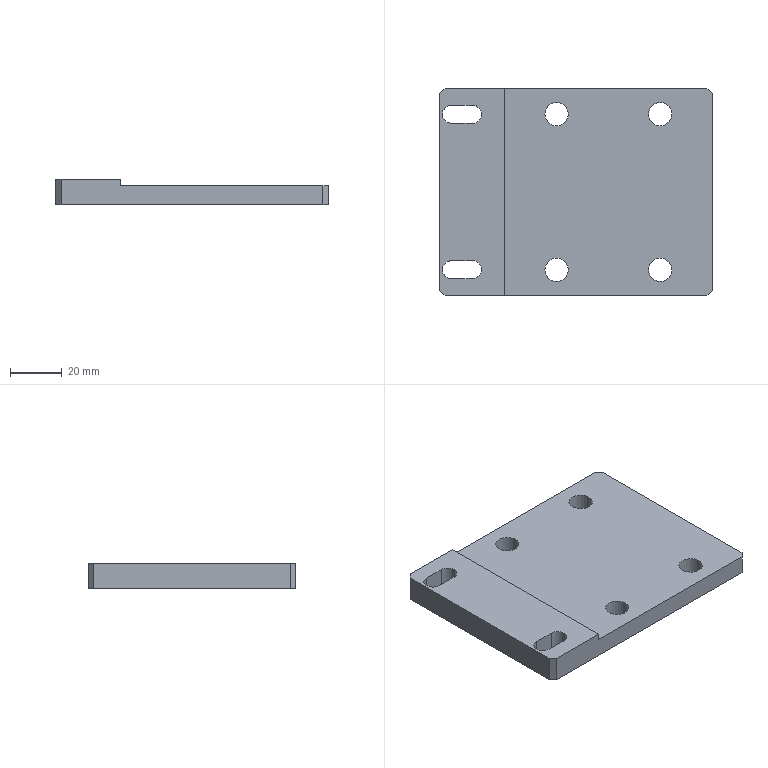Part | SolidWorks | features HoleWzd 2, ICE 2, Chamfer 1, Extrusion 1, LPattern 1 | 1 solid | 30 faces | box 105 x 80 x 10 mm | volume 64132 mm3 | plane 16 | cylinder 14 | commonest cylinder face diameters 9 x8 7 x6
STEP:
#1=CARTESIAN_POINT('',(-36.5,-30.,-5.));
#2=VERTEX_POINT('',#1);
#3=CARTESIAN_POINT('',(-40.,-26.5,-5.));
#4=VERTEX_POINT('',#3);
#5=CARTESIAN_POINT('',(-40.,-30.,-5.));
#6=DIRECTION('',(0.,0.,1.));
#7=DIRECTION('',(1.,0.,0.));
#8=AXIS2_PLACEMENT_3D('',#5,#6,#7);
#9=CIRCLE('',#8,3.5);
#10=EDGE_CURVE('',#2,#4,#9,.T.);
#11=ORIENTED_EDGE('',*,*,#10,.F.);
#12=CARTESIAN_POINT('',(-36.5,-30.,5.));
#13=VERTEX_POINT('',#12);
#14=CARTESIAN_POINT('',(-36.5,-30.,-5.));
#15=DIRECTION('',(0.,0.,1.));
#16=VECTOR('',#15,1000.);
#17=LINE('',#14,#16);
#18=EDGE_CURVE('',#2,#13,#17,.T.);
#19=ORIENTED_EDGE('',*,*,#18,.T.);
#20=CARTESIAN_POINT('',(-40.,-26.5,5.));
#21=VERTEX_POINT('',#20);
#22=CARTESIAN_POINT('',(-40.,-30.,5.));
#23=DIRECTION('',(0.,0.,1.));
#24=DIRECTION('',(1.,0.,0.));
#25=AXIS2_PLACEMENT_3D('',#22,#23,#24);
#26=CIRCLE('',#25,3.5);
#27=EDGE_CURVE('',#13,#21,#26,.T.);
#28=ORIENTED_EDGE('',*,*,#27,.T.);
#29=CARTESIAN_POINT('',(-40.,-26.5,-5.));
#30=DIRECTION('',(0.,0.,1.));
#31=VECTOR('',#30,1000.);
#32=LINE('',#29,#31);
#33=EDGE_CURVE('',#4,#21,#32,.T.);
#34=ORIENTED_EDGE('',*,*,#33,.F.);
#35=EDGE_LOOP('',(#11,#19,#28,#34));
#36=FACE_OUTER_BOUND('',#35,.T.);
#37=CARTESIAN_POINT('',(-40.,-30.,-5.));
#38=DIRECTION('',(0.,0.,1.));
#39=DIRECTION('',(1.,0.,0.));
#40=AXIS2_PLACEMENT_3D('',#37,#38,#39);
#41=CYLINDRICAL_SURFACE('',#40,3.5);
#42=ADVANCED_FACE('',(#36),#41,.F.);
#43=CARTESIAN_POINT('',(-36.5,30.,-5.));
#44=VERTEX_POINT('',#43);
#45=CARTESIAN_POINT('',(-40.,33.5,-5.));
#46=VERTEX_POINT('',#45);
#47=CARTESIAN_POINT('',(-40.,30.,-5.));
#48=DIRECTION('',(0.,0.,1.));
#49=DIRECTION('',(1.,0.,0.));
#50=AXIS2_PLACEMENT_3D('',#47,#48,#49);
#51=CIRCLE('',#50,3.5);
#52=EDGE_CURVE('',#44,#46,#51,.T.);
#53=ORIENTED_EDGE('',*,*,#52,.F.);
#54=CARTESIAN_POINT('',(-36.5,30.,5.));
#55=VERTEX_POINT('',#54);
#56=CARTESIAN_POINT('',(-36.5,30.,-5.));
#57=DIRECTION('',(0.,0.,1.));
#58=VECTOR('',#57,1000.);
#59=LINE('',#56,#58);
#60=EDGE_CURVE('',#44,#55,#59,.T.);
#61=ORIENTED_EDGE('',*,*,#60,.T.);
#62=CARTESIAN_POINT('',(-40.,33.5,5.));
#63=VERTEX_POINT('',#62);
#64=CARTESIAN_POINT('',(-40.,30.,5.));
#65=DIRECTION('',(0.,0.,1.));
#66=DIRECTION('',(1.,0.,0.));
#67=AXIS2_PLACEMENT_3D('',#64,#65,#66);
#68=CIRCLE('',#67,3.5);
#69=EDGE_CURVE('',#55,#63,#68,.T.);
#70=ORIENTED_EDGE('',*,*,#69,.T.);
#71=CARTESIAN_POINT('',(-40.,33.5,-5.));
#72=DIRECTION('',(0.,0.,1.));
#73=VECTOR('',#72,1000.);
#74=LINE('',#71,#73);
#75=EDGE_CURVE('',#46,#63,#74,.T.);
#76=ORIENTED_EDGE('',*,*,#75,.F.);
#77=EDGE_LOOP('',(#53,#61,#70,#76));
#78=FACE_OUTER_BOUND('',#77,.T.);
#79=CARTESIAN_POINT('',(-40.,30.,-5.));
#80=DIRECTION('',(0.,0.,1.));
#81=DIRECTION('',(1.,0.,0.));
#82=AXIS2_PLACEMENT_3D('',#79,#80,#81);
#83=CYLINDRICAL_SURFACE('',#82,3.5);
#84=ADVANCED_FACE('',(#78),#83,.F.);
#85=CARTESIAN_POINT('',(-12.,30.,-5.));
#86=VERTEX_POINT('',#85);
#87=CARTESIAN_POINT('',(-3.,30.,-5.));
#88=VERTEX_POINT('',#87);
#89=CARTESIAN_POINT('',(-7.5,30.,-5.));
#90=DIRECTION('',(0.,0.,1.));
#91=DIRECTION('',(1.,0.,0.));
#92=AXIS2_PLACEMENT_3D('',#89,#90,#91);
#93=CIRCLE('',#92,4.5);
#94=EDGE_CURVE('',#86,#88,#93,.T.);
#95=ORIENTED_EDGE('',*,*,#94,.F.);
#96=CARTESIAN_POINT('',(-12.,30.,2.5));
#97=VERTEX_POINT('',#96);
#98=CARTESIAN_POINT('',(-12.,30.,5.));
#99=DIRECTION('',(0.,0.,1.));
#100=VECTOR('',#99,1000.);
#101=LINE('',#98,#100);
#102=EDGE_CURVE('',#86,#97,#101,.T.);
#103=ORIENTED_EDGE('',*,*,#102,.T.);
#104=CARTESIAN_POINT('',(-3.,30.,2.5));
#105=VERTEX_POINT('',#104);
#106=CARTESIAN_POINT('',(-7.5,30.,2.5));
#107=DIRECTION('',(0.,0.,-1.));
#108=DIRECTION('',(-1.,0.,0.));
#109=AXIS2_PLACEMENT_3D('',#106,#107,#108);
#110=CIRCLE('',#109,4.5);
#111=EDGE_CURVE('',#105,#97,#110,.T.);
#112=ORIENTED_EDGE('',*,*,#111,.F.);
#113=CARTESIAN_POINT('',(-3.,30.,5.));
#114=DIRECTION('',(0.,0.,1.));
#115=VECTOR('',#114,1000.);
#116=LINE('',#113,#115);
#117=EDGE_CURVE('',#88,#105,#116,.T.);
#118=ORIENTED_EDGE('',*,*,#117,.F.);
#119=EDGE_LOOP('',(#95,#103,#112,#118));
#120=FACE_OUTER_BOUND('',#119,.T.);
#121=CARTESIAN_POINT('',(-7.5,30.,5.));
#122=DIRECTION('',(0.,0.,1.));
#123=DIRECTION('',(1.,0.,0.));
#124=AXIS2_PLACEMENT_3D('',#121,#122,#123);
#125=CYLINDRICAL_SURFACE('',#124,4.5);
#126=ADVANCED_FACE('',(#120),#125,.F.);
#127=CARTESIAN_POINT('',(28.,30.,-5.));
#128=VERTEX_POINT('',#127);
#129=CARTESIAN_POINT('',(37.,30.,-5.));
#130=VERTEX_POINT('',#129);
#131=CARTESIAN_POINT('',(32.5,30.,-5.));
#132=DIRECTION('',(0.,0.,1.));
#133=DIRECTION('',(1.,0.,0.));
#134=AXIS2_PLACEMENT_3D('',#131,#132,#133);
#135=CIRCLE('',#134,4.5);
#136=EDGE_CURVE('',#128,#130,#135,.T.);
#137=ORIENTED_EDGE('',*,*,#136,.F.);
#138=CARTESIAN_POINT('',(28.,30.,2.5));
#139=VERTEX_POINT('',#138);
#140=CARTESIAN_POINT('',(28.,30.,5.));
#141=DIRECTION('',(0.,0.,1.));
#142=VECTOR('',#141,1000.);
#143=LINE('',#140,#142);
#144=EDGE_CURVE('',#128,#139,#143,.T.);
#145=ORIENTED_EDGE('',*,*,#144,.T.);
#146=CARTESIAN_POINT('',(37.,30.,2.5));
#147=VERTEX_POINT('',#146);
#148=CARTESIAN_POINT('',(32.5,30.,2.5));
#149=DIRECTION('',(0.,0.,-1.));
#150=DIRECTION('',(-1.,0.,0.));
#151=AXIS2_PLACEMENT_3D('',#148,#149,#150);
#152=CIRCLE('',#151,4.5);
#153=EDGE_CURVE('',#147,#139,#152,.T.);
#154=ORIENTED_EDGE('',*,*,#153,.F.);
#155=CARTESIAN_POINT('',(37.,30.,5.));
#156=DIRECTION('',(0.,0.,1.));
#157=VECTOR('',#156,1000.);
#158=LINE('',#155,#157);
#159=EDGE_CURVE('',#130,#147,#158,.T.);
#160=ORIENTED_EDGE('',*,*,#159,.F.);
#161=EDGE_LOOP('',(#137,#145,#154,#160));
#162=FACE_OUTER_BOUND('',#161,.T.);
#163=CARTESIAN_POINT('',(32.5,30.,5.));
#164=DIRECTION('',(0.,0.,1.));
#165=DIRECTION('',(1.,0.,0.));
#166=AXIS2_PLACEMENT_3D('',#163,#164,#165);
#167=CYLINDRICAL_SURFACE('',#166,4.5);
#168=ADVANCED_FACE('',(#162),#167,.F.);
#169=CARTESIAN_POINT('',(28.,-30.,-5.));
#170=VERTEX_POINT('',#169);
#171=CARTESIAN_POINT('',(37.,-30.,-5.));
#172=VERTEX_POINT('',#171);
#173=CARTESIAN_POINT('',(32.5,-30.,-5.));
#174=DIRECTION('',(0.,0.,1.));
#175=DIRECTION('',(1.,0.,0.));
#176=AXIS2_PLACEMENT_3D('',#173,#174,#175);
#177=CIRCLE('',#176,4.5);
#178=EDGE_CURVE('',#170,#172,#177,.T.);
#179=ORIENTED_EDGE('',*,*,#178,.F.);
#180=CARTESIAN_POINT('',(28.,-30.,2.5));
#181=VERTEX_POINT('',#180);
#182=CARTESIAN_POINT('',(28.,-30.,5.));
#183=DIRECTION('',(0.,0.,1.));
#184=VECTOR('',#183,1000.);
#185=LINE('',#182,#184);
#186=EDGE_CURVE('',#170,#181,#185,.T.);
#187=ORIENTED_EDGE('',*,*,#186,.T.);
#188=CARTESIAN_POINT('',(37.,-30.,2.5));
#189=VERTEX_POINT('',#188);
#190=CARTESIAN_POINT('',(32.5,-30.,2.5));
#191=DIRECTION('',(0.,0.,-1.));
#192=DIRECTION('',(-1.,0.,0.));
#193=AXIS2_PLACEMENT_3D('',#190,#191,#192);
#194=CIRCLE('',#193,4.5);
#195=EDGE_CURVE('',#189,#181,#194,.T.);
#196=ORIENTED_EDGE('',*,*,#195,.F.);
#197=CARTESIAN_POINT('',(37.,-30.,5.));
#198=DIRECTION('',(0.,0.,1.));
#199=VECTOR('',#198,1000.);
#200=LINE('',#197,#199);
#201=EDGE_CURVE('',#172,#189,#200,.T.);
#202=ORIENTED_EDGE('',*,*,#201,.F.);
#203=EDGE_LOOP('',(#179,#187,#196,#202));
#204=FACE_OUTER_BOUND('',#203,.T.);
#205=CARTESIAN_POINT('',(32.5,-30.,5.));
#206=DIRECTION('',(0.,0.,1.));
#207=DIRECTION('',(1.,0.,0.));
#208=AXIS2_PLACEMENT_3D('',#205,#206,#207);
#209=CYLINDRICAL_SURFACE('',#208,4.5);
#210=ADVANCED_FACE('',(#204),#209,.F.);
#211=CARTESIAN_POINT('',(-12.,-30.,-5.));
#212=VERTEX_POINT('',#211);
#213=CARTESIAN_POINT('',(-3.,-30.,-5.));
#214=VERTEX_POINT('',#213);
#215=CARTESIAN_POINT('',(-7.5,-30.,-5.));
#216=DIRECTION('',(0.,0.,1.));
#217=DIRECTION('',(1.,0.,0.));
#218=AXIS2_PLACEMENT_3D('',#215,#216,#217);
#219=CIRCLE('',#218,4.5);
#220=EDGE_CURVE('',#212,#214,#219,.T.);
#221=ORIENTED_EDGE('',*,*,#220,.F.);
#222=CARTESIAN_POINT('',(-12.,-30.,2.5));
#223=VERTEX_POINT('',#222);
#224=CARTESIAN_POINT('',(-12.,-30.,5.));
#225=DIRECTION('',(0.,0.,1.));
#226=VECTOR('',#225,1000.);
#227=LINE('',#224,#226);
#228=EDGE_CURVE('',#212,#223,#227,.T.);
#229=ORIENTED_EDGE('',*,*,#228,.T.);
#230=CARTESIAN_POINT('',(-3.,-30.,2.5));
#231=VERTEX_POINT('',#230);
#232=CARTESIAN_POINT('',(-7.5,-30.,2.5));
#233=DIRECTION('',(0.,0.,-1.));
#234=DIRECTION('',(-1.,0.,0.));
#235=AXIS2_PLACEMENT_3D('',#232,#233,#234);
#236=CIRCLE('',#235,4.5);
#237=EDGE_CURVE('',#231,#223,#236,.T.);
#238=ORIENTED_EDGE('',*,*,#237,.F.);
#239=CARTESIAN_POINT('',(-3.,-30.,5.));
#240=DIRECTION('',(0.,0.,1.));
#241=VECTOR('',#240,1000.);
#242=LINE('',#239,#241);
#243=EDGE_CURVE('',#214,#231,#242,.T.);
#244=ORIENTED_EDGE('',*,*,#243,.F.);
#245=EDGE_LOOP('',(#221,#229,#238,#244));
#246=FACE_OUTER_BOUND('',#245,.T.);
#247=CARTESIAN_POINT('',(-7.5,-30.,5.));
#248=DIRECTION('',(0.,0.,1.));
#249=DIRECTION('',(1.,0.,0.));
#250=AXIS2_PLACEMENT_3D('',#247,#248,#249);
#251=CYLINDRICAL_SURFACE('',#250,4.5);
#252=ADVANCED_FACE('',(#246),#251,.F.);
#253=CARTESIAN_POINT('',(52.5,-38.,-5.));
#254=VERTEX_POINT('',#253);
#255=CARTESIAN_POINT('',(52.5,38.,-5.));
#256=VERTEX_POINT('',#255);
#257=CARTESIAN_POINT('',(52.5,40.,-5.));
#258=DIRECTION('',(0.,1.,0.));
#259=VECTOR('',#258,1000.);
#260=LINE('',#257,#259);
#261=EDGE_CURVE('',#254,#256,#260,.T.);
#262=ORIENTED_EDGE('',*,*,#261,.T.);
#263=CARTESIAN_POINT('',(52.5,38.,2.5));
#264=VERTEX_POINT('',#263);
#265=CARTESIAN_POINT('',(52.5,38.,5.));
#266=DIRECTION('',(0.,0.,1.));
#267=VECTOR('',#266,1000.);
#268=LINE('',#265,#267);
#269=EDGE_CURVE('',#256,#264,#268,.T.);
#270=ORIENTED_EDGE('',*,*,#269,.T.);
#271=CARTESIAN_POINT('',(52.5,-38.,2.5));
#272=VERTEX_POINT('',#271);
#273=CARTESIAN_POINT('',(52.5,40.,2.5));
#274=DIRECTION('',(0.,1.,0.));
#275=VECTOR('',#274,1000.);
#276=LINE('',#273,#275);
#277=EDGE_CURVE('',#272,#264,#276,.T.);
#278=ORIENTED_EDGE('',*,*,#277,.F.);
#279=CARTESIAN_POINT('',(52.5,-38.,5.));
#280=DIRECTION('',(0.,0.,-1.));
#281=VECTOR('',#280,1000.);
#282=LINE('',#279,#281);
#283=EDGE_CURVE('',#272,#254,#282,.T.);
#284=ORIENTED_EDGE('',*,*,#283,.T.);
#285=EDGE_LOOP('',(#262,#270,#278,#284));
#286=FACE_OUTER_BOUND('',#285,.T.);
#287=CARTESIAN_POINT('',(52.5,40.,5.));
#288=DIRECTION('',(-1.,0.,0.));
#289=DIRECTION('',(0.,-1.,0.));
#290=AXIS2_PLACEMENT_3D('',#287,#288,#289);
#291=PLANE('',#290);
#292=ADVANCED_FACE('',(#286),#291,.F.);
#293=CARTESIAN_POINT('',(50.5,40.,-5.));
#294=VERTEX_POINT('',#293);
#295=CARTESIAN_POINT('',(-50.5,40.,-5.));
#296=VERTEX_POINT('',#295);
#297=CARTESIAN_POINT('',(-52.5,40.,-5.));
#298=DIRECTION('',(-1.,0.,0.));
#299=VECTOR('',#298,1000.);
#300=LINE('',#297,#299);
#301=EDGE_CURVE('',#294,#296,#300,.T.);
#302=ORIENTED_EDGE('',*,*,#301,.T.);
#303=CARTESIAN_POINT('',(-50.5,40.,5.));
#304=VERTEX_POINT('',#303);
#305=CARTESIAN_POINT('',(-50.5,40.,5.));
#306=DIRECTION('',(0.,0.,1.));
#307=VECTOR('',#306,1000.);
#308=LINE('',#305,#307);
#309=EDGE_CURVE('',#296,#304,#308,.T.);
#310=ORIENTED_EDGE('',*,*,#309,.T.);
#311=CARTESIAN_POINT('',(-27.5,40.,5.));
#312=VERTEX_POINT('',#311);
#313=CARTESIAN_POINT('',(-52.5,40.,5.));
#314=DIRECTION('',(-1.,0.,0.));
#315=VECTOR('',#314,1000.);
#316=LINE('',#313,#315);
#317=EDGE_CURVE('',#312,#304,#316,.T.);
#318=ORIENTED_EDGE('',*,*,#317,.F.);
#319=CARTESIAN_POINT('',(-27.5,40.,2.5));
#320=VERTEX_POINT('',#319);
#321=CARTESIAN_POINT('',(-27.5,40.,2.5));
#322=DIRECTION('',(0.,0.,1.));
#323=VECTOR('',#322,1000.);
#324=LINE('',#321,#323);
#325=EDGE_CURVE('',#320,#312,#324,.T.);
#326=ORIENTED_EDGE('',*,*,#325,.F.);
#327=CARTESIAN_POINT('',(50.5,40.,2.5));
#328=VERTEX_POINT('',#327);
#329=CARTESIAN_POINT('',(52.5,40.,2.5));
#330=DIRECTION('',(-1.,0.,0.));
#331=VECTOR('',#330,1000.);
#332=LINE('',#329,#331);
#333=EDGE_CURVE('',#328,#320,#332,.T.);
#334=ORIENTED_EDGE('',*,*,#333,.F.);
#335=CARTESIAN_POINT('',(50.5,40.,5.));
#336=DIRECTION('',(0.,0.,-1.));
#337=VECTOR('',#336,1000.);
#338=LINE('',#335,#337);
#339=EDGE_CURVE('',#328,#294,#338,.T.);
#340=ORIENTED_EDGE('',*,*,#339,.T.);
#341=EDGE_LOOP('',(#302,#310,#318,#326,#334,#340));
#342=FACE_OUTER_BOUND('',#341,.T.);
#343=CARTESIAN_POINT('',(-52.5,40.,5.));
#344=DIRECTION('',(0.,-1.,0.));
#345=DIRECTION('',(0.,0.,-1.));
#346=AXIS2_PLACEMENT_3D('',#343,#344,#345);
#347=PLANE('',#346);
#348=ADVANCED_FACE('',(#342),#347,.F.);
#349=CARTESIAN_POINT('',(-52.5,38.,-5.));
#350=VERTEX_POINT('',#349);
#351=CARTESIAN_POINT('',(-52.5,-38.,-5.));
#352=VERTEX_POINT('',#351);
#353=CARTESIAN_POINT('',(-52.5,40.,-5.));
#354=DIRECTION('',(0.,-1.,0.));
#355=VECTOR('',#354,1000.);
#356=LINE('',#353,#355);
#357=EDGE_CURVE('',#350,#352,#356,.T.);
#358=ORIENTED_EDGE('',*,*,#357,.T.);
#359=CARTESIAN_POINT('',(-52.5,-38.,5.));
#360=VERTEX_POINT('',#359);
#361=CARTESIAN_POINT('',(-52.5,-38.,5.));
#362=DIRECTION('',(0.,0.,1.));
#363=VECTOR('',#362,1000.);
#364=LINE('',#361,#363);
#365=EDGE_CURVE('',#352,#360,#364,.T.);
#366=ORIENTED_EDGE('',*,*,#365,.T.);
#367=CARTESIAN_POINT('',(-52.5,38.,5.));
#368=VERTEX_POINT('',#367);
#369=CARTESIAN_POINT('',(-52.5,40.,5.));
#370=DIRECTION('',(0.,-1.,0.));
#371=VECTOR('',#370,1000.);
#372=LINE('',#369,#371);
#373=EDGE_CURVE('',#368,#360,#372,.T.);
#374=ORIENTED_EDGE('',*,*,#373,.F.);
#375=CARTESIAN_POINT('',(-52.5,38.,5.));
#376=DIRECTION('',(0.,0.,-1.));
#377=VECTOR('',#376,1000.);
#378=LINE('',#375,#377);
#379=EDGE_CURVE('',#368,#350,#378,.T.);
#380=ORIENTED_EDGE('',*,*,#379,.T.);
#381=EDGE_LOOP('',(#358,#366,#374,#380));
#382=FACE_OUTER_BOUND('',#381,.T.);
#383=CARTESIAN_POINT('',(-52.5,40.,5.));
#384=DIRECTION('',(1.,0.,0.));
#385=DIRECTION('',(0.,1.,0.));
#386=AXIS2_PLACEMENT_3D('',#383,#384,#385);
#387=PLANE('',#386);
#388=ADVANCED_FACE('',(#382),#387,.F.);
#389=CARTESIAN_POINT('',(-50.5,-40.,5.));
#390=VERTEX_POINT('',#389);
#391=CARTESIAN_POINT('',(-27.5,-40.,5.));
#392=VERTEX_POINT('',#391);
#393=CARTESIAN_POINT('',(-52.5,-40.,5.));
#394=DIRECTION('',(1.,0.,0.));
#395=VECTOR('',#394,1000.);
#396=LINE('',#393,#395);
#397=EDGE_CURVE('',#390,#392,#396,.T.);
#398=ORIENTED_EDGE('',*,*,#397,.F.);
#399=CARTESIAN_POINT('',(-50.5,-40.,-5.));
#400=VERTEX_POINT('',#399);
#401=CARTESIAN_POINT('',(-50.5,-40.,5.));
#402=DIRECTION('',(0.,0.,-1.));
#403=VECTOR('',#402,1000.);
#404=LINE('',#401,#403);
#405=EDGE_CURVE('',#390,#400,#404,.T.);
#406=ORIENTED_EDGE('',*,*,#405,.T.);
#407=CARTESIAN_POINT('',(50.5,-40.,-5.));
#408=VERTEX_POINT('',#407);
#409=CARTESIAN_POINT('',(-52.5,-40.,-5.));
#410=DIRECTION('',(1.,0.,0.));
#411=VECTOR('',#410,1000.);
#412=LINE('',#409,#411);
#413=EDGE_CURVE('',#400,#408,#412,.T.);
#414=ORIENTED_EDGE('',*,*,#413,.T.);
#415=CARTESIAN_POINT('',(50.5,-40.,2.5));
#416=VERTEX_POINT('',#415);
#417=CARTESIAN_POINT('',(50.5,-40.,5.));
#418=DIRECTION('',(0.,0.,1.));
#419=VECTOR('',#418,1000.);
#420=LINE('',#417,#419);
#421=EDGE_CURVE('',#408,#416,#420,.T.);
#422=ORIENTED_EDGE('',*,*,#421,.T.);
#423=CARTESIAN_POINT('',(-27.5,-40.,2.5));
#424=VERTEX_POINT('',#423);
#425=CARTESIAN_POINT('',(52.5,-40.,2.5));
#426=DIRECTION('',(1.,0.,0.));
#427=VECTOR('',#426,1000.);
#428=LINE('',#425,#427);
#429=EDGE_CURVE('',#424,#416,#428,.T.);
#430=ORIENTED_EDGE('',*,*,#429,.F.);
#431=CARTESIAN_POINT('',(-27.5,-40.,2.5));
#432=DIRECTION('',(0.,0.,1.));
#433=VECTOR('',#432,1000.);
#434=LINE('',#431,#433);
#435=EDGE_CURVE('',#424,#392,#434,.T.);
#436=ORIENTED_EDGE('',*,*,#435,.T.);
#437=EDGE_LOOP('',(#398,#406,#414,#422,#430,#436));
#438=FACE_OUTER_BOUND('',#437,.T.);
#439=CARTESIAN_POINT('',(-52.5,-40.,5.));
#440=DIRECTION('',(0.,1.,0.));
#441=DIRECTION('',(0.,0.,1.));
#442=AXIS2_PLACEMENT_3D('',#439,#440,#441);
#443=PLANE('',#442);
#444=ADVANCED_FACE('',(#438),#443,.F.);
#445=CARTESIAN_POINT('',(-40.,-33.5,5.));
#446=VERTEX_POINT('',#445);
#447=CARTESIAN_POINT('',(-40.,-30.,5.));
#448=DIRECTION('',(0.,0.,1.));
#449=DIRECTION('',(1.,0.,0.));
#450=AXIS2_PLACEMENT_3D('',#447,#448,#449);
#451=CIRCLE('',#450,3.5);
#452=EDGE_CURVE('',#446,#13,#451,.T.);
#453=ORIENTED_EDGE('',*,*,#452,.F.);
#454=CARTESIAN_POINT('',(-48.,-33.5,5.));
#455=VERTEX_POINT('',#454);
#456=CARTESIAN_POINT('',(-40.,-33.5,5.));
#457=DIRECTION('',(1.,0.,0.));
#458=VECTOR('',#457,1000.);
#459=LINE('',#456,#458);
#460=EDGE_CURVE('',#455,#446,#459,.T.);
#461=ORIENTED_EDGE('',*,*,#460,.F.);
#462=CARTESIAN_POINT('',(-48.,-26.5,5.));
#463=VERTEX_POINT('',#462);
#464=CARTESIAN_POINT('',(-48.,-30.,5.));
#465=DIRECTION('',(0.,0.,1.));
#466=DIRECTION('',(1.,0.,0.));
#467=AXIS2_PLACEMENT_3D('',#464,#465,#466);
#468=CIRCLE('',#467,3.5);
#469=EDGE_CURVE('',#463,#455,#468,.T.);
#470=ORIENTED_EDGE('',*,*,#469,.F.);
#471=CARTESIAN_POINT('',(-40.,-26.5,5.));
#472=DIRECTION('',(-1.,0.,0.));
#473=VECTOR('',#472,1000.);
#474=LINE('',#471,#473);
#475=EDGE_CURVE('',#21,#463,#474,.T.);
#476=ORIENTED_EDGE('',*,*,#475,.F.);
#477=ORIENTED_EDGE('',*,*,#27,.F.);
#478=EDGE_LOOP('',(#453,#461,#470,#476,#477));
#479=FACE_BOUND('',#478,.T.);
#480=CARTESIAN_POINT('',(-40.,26.5,5.));
#481=VERTEX_POINT('',#480);
#482=CARTESIAN_POINT('',(-40.,30.,5.));
#483=DIRECTION('',(0.,0.,1.));
#484=DIRECTION('',(1.,0.,0.));
#485=AXIS2_PLACEMENT_3D('',#482,#483,#484);
#486=CIRCLE('',#485,3.5);
#487=EDGE_CURVE('',#481,#55,#486,.T.);
#488=ORIENTED_EDGE('',*,*,#487,.F.);
#489=CARTESIAN_POINT('',(-48.,26.5,5.));
#490=VERTEX_POINT('',#489);
#491=CARTESIAN_POINT('',(-40.,26.5,5.));
#492=DIRECTION('',(1.,0.,0.));
#493=VECTOR('',#492,1000.);
#494=LINE('',#491,#493);
#495=EDGE_CURVE('',#490,#481,#494,.T.);
#496=ORIENTED_EDGE('',*,*,#495,.F.);
#497=CARTESIAN_POINT('',(-48.,33.5,5.));
#498=VERTEX_POINT('',#497);
#499=CARTESIAN_POINT('',(-48.,30.,5.));
#500=DIRECTION('',(0.,0.,1.));
#501=DIRECTION('',(1.,0.,0.));
#502=AXIS2_PLACEMENT_3D('',#499,#500,#501);
#503=CIRCLE('',#502,3.5);
#504=EDGE_CURVE('',#498,#490,#503,.T.);
#505=ORIENTED_EDGE('',*,*,#504,.F.);
#506=CARTESIAN_POINT('',(-40.,33.5,5.));
#507=DIRECTION('',(-1.,0.,0.));
#508=VECTOR('',#507,1000.);
#509=LINE('',#506,#508);
#510=EDGE_CURVE('',#63,#498,#509,.T.);
#511=ORIENTED_EDGE('',*,*,#510,.F.);
#512=ORIENTED_EDGE('',*,*,#69,.F.);
#513=EDGE_LOOP('',(#488,#496,#505,#511,#512));
#514=FACE_BOUND('',#513,.T.);
#515=ORIENTED_EDGE('',*,*,#373,.T.);
#516=CARTESIAN_POINT('',(-45.25,-45.25,5.));
#517=DIRECTION('',(0.7071,-0.7071,0.));
#518=VECTOR('',#517,1000.);
#519=LINE('',#516,#518);
#520=EDGE_CURVE('',#360,#390,#519,.T.);
#521=ORIENTED_EDGE('',*,*,#520,.T.);
#522=ORIENTED_EDGE('',*,*,#397,.T.);
#523=CARTESIAN_POINT('',(-27.5,40.,5.));
#524=DIRECTION('',(0.,-1.,0.));
#525=VECTOR('',#524,1000.);
#526=LINE('',#523,#525);
#527=EDGE_CURVE('',#312,#392,#526,.T.);
#528=ORIENTED_EDGE('',*,*,#527,.F.);
#529=ORIENTED_EDGE('',*,*,#317,.T.);
#530=CARTESIAN_POINT('',(-45.25,45.25,5.));
#531=DIRECTION('',(-0.7071,-0.7071,0.));
#532=VECTOR('',#531,1000.);
#533=LINE('',#530,#532);
#534=EDGE_CURVE('',#304,#368,#533,.T.);
#535=ORIENTED_EDGE('',*,*,#534,.T.);
#536=EDGE_LOOP('',(#515,#521,#522,#528,#529,#535));
#537=FACE_OUTER_BOUND('',#536,.T.);
#538=CARTESIAN_POINT('',(0.,0.,5.));
#539=DIRECTION('',(0.,0.,1.));
#540=DIRECTION('',(1.,0.,0.));
#541=AXIS2_PLACEMENT_3D('',#538,#539,#540);
#542=PLANE('',#541);
#543=ADVANCED_FACE('',(#479,#514,#537),#542,.T.);
#544=CARTESIAN_POINT('',(-48.,33.5,-5.));
#545=VERTEX_POINT('',#544);
#546=CARTESIAN_POINT('',(-48.,26.5,-5.));
#547=VERTEX_POINT('',#546);
#548=CARTESIAN_POINT('',(-48.,30.,-5.));
#549=DIRECTION('',(0.,0.,1.));
#550=DIRECTION('',(1.,0.,0.));
#551=AXIS2_PLACEMENT_3D('',#548,#549,#550);
#552=CIRCLE('',#551,3.5);
#553=EDGE_CURVE('',#545,#547,#552,.T.);
#554=ORIENTED_EDGE('',*,*,#553,.T.);
#555=CARTESIAN_POINT('',(-40.,26.5,-5.));
#556=VERTEX_POINT('',#555);
#557=CARTESIAN_POINT('',(-40.,26.5,-5.));
#558=DIRECTION('',(1.,0.,0.));
#559=VECTOR('',#558,1000.);
#560=LINE('',#557,#559);
#561=EDGE_CURVE('',#547,#556,#560,.T.);
#562=ORIENTED_EDGE('',*,*,#561,.T.);
#563=CARTESIAN_POINT('',(-40.,30.,-5.));
#564=DIRECTION('',(0.,0.,1.));
#565=DIRECTION('',(1.,0.,0.));
#566=AXIS2_PLACEMENT_3D('',#563,#564,#565);
#567=CIRCLE('',#566,3.5);
#568=EDGE_CURVE('',#556,#44,#567,.T.);
#569=ORIENTED_EDGE('',*,*,#568,.T.);
#570=ORIENTED_EDGE('',*,*,#52,.T.);
#571=CARTESIAN_POINT('',(-40.,33.5,-5.));
#572=DIRECTION('',(-1.,0.,0.));
#573=VECTOR('',#572,1000.);
#574=LINE('',#571,#573);
#575=EDGE_CURVE('',#46,#545,#574,.T.);
#576=ORIENTED_EDGE('',*,*,#575,.T.);
#577=EDGE_LOOP('',(#554,#562,#569,#570,#576));
#578=FACE_BOUND('',#577,.T.);
#579=CARTESIAN_POINT('',(-48.,-26.5,-5.));
#580=VERTEX_POINT('',#579);
#581=CARTESIAN_POINT('',(-48.,-33.5,-5.));
#582=VERTEX_POINT('',#581);
#583=CARTESIAN_POINT('',(-48.,-30.,-5.));
#584=DIRECTION('',(0.,0.,1.));
#585=DIRECTION('',(1.,0.,0.));
#586=AXIS2_PLACEMENT_3D('',#583,#584,#585);
#587=CIRCLE('',#586,3.5);
#588=EDGE_CURVE('',#580,#582,#587,.T.);
#589=ORIENTED_EDGE('',*,*,#588,.T.);
#590=CARTESIAN_POINT('',(-40.,-33.5,-5.));
#591=VERTEX_POINT('',#590);
#592=CARTESIAN_POINT('',(-40.,-33.5,-5.));
#593=DIRECTION('',(1.,0.,0.));
#594=VECTOR('',#593,1000.);
#595=LINE('',#592,#594);
#596=EDGE_CURVE('',#582,#591,#595,.T.);
#597=ORIENTED_EDGE('',*,*,#596,.T.);
#598=CARTESIAN_POINT('',(-40.,-30.,-5.));
#599=DIRECTION('',(0.,0.,1.));
#600=DIRECTION('',(1.,0.,0.));
#601=AXIS2_PLACEMENT_3D('',#598,#599,#600);
#602=CIRCLE('',#601,3.5);
#603=EDGE_CURVE('',#591,#2,#602,.T.);
#604=ORIENTED_EDGE('',*,*,#603,.T.);
#605=ORIENTED_EDGE('',*,*,#10,.T.);
#606=CARTESIAN_POINT('',(-40.,-26.5,-5.));
#607=DIRECTION('',(-1.,0.,0.));
#608=VECTOR('',#607,1000.);
#609=LINE('',#606,#608);
#610=EDGE_CURVE('',#4,#580,#609,.T.);
#611=ORIENTED_EDGE('',*,*,#610,.T.);
#612=EDGE_LOOP('',(#589,#597,#604,#605,#611));
#613=FACE_BOUND('',#612,.T.);
#614=CARTESIAN_POINT('',(-7.5,30.,-5.));
#615=DIRECTION('',(0.,0.,1.));
#616=DIRECTION('',(1.,0.,0.));
#617=AXIS2_PLACEMENT_3D('',#614,#615,#616);
#618=CIRCLE('',#617,4.5);
#619=EDGE_CURVE('',#88,#86,#618,.T.);
#620=ORIENTED_EDGE('',*,*,#619,.T.);
#621=ORIENTED_EDGE('',*,*,#94,.T.);
#622=EDGE_LOOP('',(#620,#621));
#623=FACE_BOUND('',#622,.T.);
#624=CARTESIAN_POINT('',(32.5,30.,-5.));
#625=DIRECTION('',(0.,0.,1.));
#626=DIRECTION('',(1.,0.,0.));
#627=AXIS2_PLACEMENT_3D('',#624,#625,#626);
#628=CIRCLE('',#627,4.5);
#629=EDGE_CURVE('',#130,#128,#628,.T.);
#630=ORIENTED_EDGE('',*,*,#629,.T.);
#631=ORIENTED_EDGE('',*,*,#136,.T.);
#632=EDGE_LOOP('',(#630,#631));
#633=FACE_BOUND('',#632,.T.);
#634=CARTESIAN_POINT('',(32.5,-30.,-5.));
#635=DIRECTION('',(0.,0.,1.));
#636=DIRECTION('',(1.,0.,0.));
#637=AXIS2_PLACEMENT_3D('',#634,#635,#636);
#638=CIRCLE('',#637,4.5);
#639=EDGE_CURVE('',#172,#170,#638,.T.);
#640=ORIENTED_EDGE('',*,*,#639,.T.);
#641=ORIENTED_EDGE('',*,*,#178,.T.);
#642=EDGE_LOOP('',(#640,#641));
#643=FACE_BOUND('',#642,.T.);
#644=CARTESIAN_POINT('',(-7.5,-30.,-5.));
#645=DIRECTION('',(0.,0.,1.));
#646=DIRECTION('',(1.,0.,0.));
#647=AXIS2_PLACEMENT_3D('',#644,#645,#646);
#648=CIRCLE('',#647,4.5);
#649=EDGE_CURVE('',#214,#212,#648,.T.);
#650=ORIENTED_EDGE('',*,*,#649,.T.);
#651=ORIENTED_EDGE('',*,*,#220,.T.);
#652=EDGE_LOOP('',(#650,#651));
#653=FACE_BOUND('',#652,.T.);
#654=ORIENTED_EDGE('',*,*,#413,.F.);
#655=CARTESIAN_POINT('',(-50.5,-40.,-5.));
#656=DIRECTION('',(-0.7071,0.7071,0.));
#657=VECTOR('',#656,1000.);
#658=LINE('',#655,#657);
#659=EDGE_CURVE('',#400,#352,#658,.T.);
#660=ORIENTED_EDGE('',*,*,#659,.T.);
#661=ORIENTED_EDGE('',*,*,#357,.F.);
#662=CARTESIAN_POINT('',(-52.5,38.,-5.));
#663=DIRECTION('',(0.7071,0.7071,0.));
#664=VECTOR('',#663,1000.);
#665=LINE('',#662,#664);
#666=EDGE_CURVE('',#350,#296,#665,.T.);
#667=ORIENTED_EDGE('',*,*,#666,.T.);
#668=ORIENTED_EDGE('',*,*,#301,.F.);
#669=CARTESIAN_POINT('',(50.5,40.,-5.));
#670=DIRECTION('',(0.7071,-0.7071,0.));
#671=VECTOR('',#670,1000.);
#672=LINE('',#669,#671);
#673=EDGE_CURVE('',#294,#256,#672,.T.);
#674=ORIENTED_EDGE('',*,*,#673,.T.);
#675=ORIENTED_EDGE('',*,*,#261,.F.);
#676=CARTESIAN_POINT('',(52.5,-38.,-5.));
#677=DIRECTION('',(-0.7071,-0.7071,0.));
#678=VECTOR('',#677,1000.);
#679=LINE('',#676,#678);
#680=EDGE_CURVE('',#254,#408,#679,.T.);
#681=ORIENTED_EDGE('',*,*,#680,.T.);
#682=EDGE_LOOP('',(#654,#660,#661,#667,#668,#674,#675,#681));
#683=FACE_OUTER_BOUND('',#682,.T.);
#684=CARTESIAN_POINT('',(0.,0.,-5.));
#685=DIRECTION('',(0.,0.,1.));
#686=DIRECTION('',(1.,0.,0.));
#687=AXIS2_PLACEMENT_3D('',#684,#685,#686);
#688=PLANE('',#687);
#689=ADVANCED_FACE('',(#578,#613,#623,#633,#643,#653,#683),#688,.F.);
#690=ORIENTED_EDGE('',*,*,#527,.T.);
#691=ORIENTED_EDGE('',*,*,#435,.F.);
#692=CARTESIAN_POINT('',(-27.5,40.,2.5));
#693=DIRECTION('',(0.,-1.,0.));
#694=VECTOR('',#693,1000.);
#695=LINE('',#692,#694);
#696=EDGE_CURVE('',#320,#424,#695,.T.);
#697=ORIENTED_EDGE('',*,*,#696,.F.);
#698=ORIENTED_EDGE('',*,*,#325,.T.);
#699=EDGE_LOOP('',(#690,#691,#697,#698));
#700=FACE_OUTER_BOUND('',#699,.T.);
#701=CARTESIAN_POINT('',(-27.5,40.,2.5));
#702=DIRECTION('',(-1.,0.,0.));
#703=DIRECTION('',(0.,-1.,0.));
#704=AXIS2_PLACEMENT_3D('',#701,#702,#703);
#705=PLANE('',#704);
#706=ADVANCED_FACE('',(#700),#705,.F.);
#707=ORIENTED_EDGE('',*,*,#111,.T.);
#708=CARTESIAN_POINT('',(-7.5,30.,2.5));
#709=DIRECTION('',(0.,0.,-1.));
#710=DIRECTION('',(-1.,0.,0.));
#711=AXIS2_PLACEMENT_3D('',#708,#709,#710);
#712=CIRCLE('',#711,4.5);
#713=EDGE_CURVE('',#97,#105,#712,.T.);
#714=ORIENTED_EDGE('',*,*,#713,.T.);
#715=EDGE_LOOP('',(#707,#714));
#716=FACE_BOUND('',#715,.T.);
#717=ORIENTED_EDGE('',*,*,#153,.T.);
#718=CARTESIAN_POINT('',(32.5,30.,2.5));
#719=DIRECTION('',(0.,0.,-1.));
#720=DIRECTION('',(-1.,0.,0.));
#721=AXIS2_PLACEMENT_3D('',#718,#719,#720);
#722=CIRCLE('',#721,4.5);
#723=EDGE_CURVE('',#139,#147,#722,.T.);
#724=ORIENTED_EDGE('',*,*,#723,.T.);
#725=EDGE_LOOP('',(#717,#724));
#726=FACE_BOUND('',#725,.T.);
#727=ORIENTED_EDGE('',*,*,#195,.T.);
#728=CARTESIAN_POINT('',(32.5,-30.,2.5));
#729=DIRECTION('',(0.,0.,-1.));
#730=DIRECTION('',(-1.,0.,0.));
#731=AXIS2_PLACEMENT_3D('',#728,#729,#730);
#732=CIRCLE('',#731,4.5);
#733=EDGE_CURVE('',#181,#189,#732,.T.);
#734=ORIENTED_EDGE('',*,*,#733,.T.);
#735=EDGE_LOOP('',(#727,#734));
#736=FACE_BOUND('',#735,.T.);
#737=ORIENTED_EDGE('',*,*,#237,.T.);
#738=CARTESIAN_POINT('',(-7.5,-30.,2.5));
#739=DIRECTION('',(0.,0.,-1.));
#740=DIRECTION('',(-1.,0.,0.));
#741=AXIS2_PLACEMENT_3D('',#738,#739,#740);
#742=CIRCLE('',#741,4.5);
#743=EDGE_CURVE('',#223,#231,#742,.T.);
#744=ORIENTED_EDGE('',*,*,#743,.T.);
#745=EDGE_LOOP('',(#737,#744));
#746=FACE_BOUND('',#745,.T.);
#747=ORIENTED_EDGE('',*,*,#277,.T.);
#748=CARTESIAN_POINT('',(50.5,40.,2.5));
#749=DIRECTION('',(-0.7071,0.7071,0.));
#750=VECTOR('',#749,1000.);
#751=LINE('',#748,#750);
#752=EDGE_CURVE('',#264,#328,#751,.T.);
#753=ORIENTED_EDGE('',*,*,#752,.T.);
#754=ORIENTED_EDGE('',*,*,#333,.T.);
#755=ORIENTED_EDGE('',*,*,#696,.T.);
#756=ORIENTED_EDGE('',*,*,#429,.T.);
#757=CARTESIAN_POINT('',(52.5,-38.,2.5));
#758=DIRECTION('',(0.7071,0.7071,0.));
#759=VECTOR('',#758,1000.);
#760=LINE('',#757,#759);
#761=EDGE_CURVE('',#416,#272,#760,.T.);
#762=ORIENTED_EDGE('',*,*,#761,.T.);
#763=EDGE_LOOP('',(#747,#753,#754,#755,#756,#762));
#764=FACE_OUTER_BOUND('',#763,.T.);
#765=CARTESIAN_POINT('',(0.,0.,2.5));
#766=DIRECTION('',(0.,0.,-1.));
#767=DIRECTION('',(-1.,0.,0.));
#768=AXIS2_PLACEMENT_3D('',#765,#766,#767);
#769=PLANE('',#768);
#770=ADVANCED_FACE('',(#716,#726,#736,#746,#764),#769,.F.);
#771=ORIENTED_EDGE('',*,*,#228,.F.);
#772=ORIENTED_EDGE('',*,*,#649,.F.);
#773=ORIENTED_EDGE('',*,*,#243,.T.);
#774=ORIENTED_EDGE('',*,*,#743,.F.);
#775=EDGE_LOOP('',(#771,#772,#773,#774));
#776=FACE_OUTER_BOUND('',#775,.T.);
#777=CARTESIAN_POINT('',(-7.5,-30.,5.));
#778=DIRECTION('',(0.,0.,1.));
#779=DIRECTION('',(1.,0.,0.));
#780=AXIS2_PLACEMENT_3D('',#777,#778,#779);
#781=CYLINDRICAL_SURFACE('',#780,4.5);
#782=ADVANCED_FACE('',(#776),#781,.F.);
#783=ORIENTED_EDGE('',*,*,#186,.F.);
#784=ORIENTED_EDGE('',*,*,#639,.F.);
#785=ORIENTED_EDGE('',*,*,#201,.T.);
#786=ORIENTED_EDGE('',*,*,#733,.F.);
#787=EDGE_LOOP('',(#783,#784,#785,#786));
#788=FACE_OUTER_BOUND('',#787,.T.);
#789=CARTESIAN_POINT('',(32.5,-30.,5.));
#790=DIRECTION('',(0.,0.,1.));
#791=DIRECTION('',(1.,0.,0.));
#792=AXIS2_PLACEMENT_3D('',#789,#790,#791);
#793=CYLINDRICAL_SURFACE('',#792,4.5);
#794=ADVANCED_FACE('',(#788),#793,.F.);
#795=ORIENTED_EDGE('',*,*,#144,.F.);
#796=ORIENTED_EDGE('',*,*,#629,.F.);
#797=ORIENTED_EDGE('',*,*,#159,.T.);
#798=ORIENTED_EDGE('',*,*,#723,.F.);
#799=EDGE_LOOP('',(#795,#796,#797,#798));
#800=FACE_OUTER_BOUND('',#799,.T.);
#801=CARTESIAN_POINT('',(32.5,30.,5.));
#802=DIRECTION('',(0.,0.,1.));
#803=DIRECTION('',(1.,0.,0.));
#804=AXIS2_PLACEMENT_3D('',#801,#802,#803);
#805=CYLINDRICAL_SURFACE('',#804,4.5);
#806=ADVANCED_FACE('',(#800),#805,.F.);
#807=ORIENTED_EDGE('',*,*,#102,.F.);
#808=ORIENTED_EDGE('',*,*,#619,.F.);
#809=ORIENTED_EDGE('',*,*,#117,.T.);
#810=ORIENTED_EDGE('',*,*,#713,.F.);
#811=EDGE_LOOP('',(#807,#808,#809,#810));
#812=FACE_OUTER_BOUND('',#811,.T.);
#813=CARTESIAN_POINT('',(-7.5,30.,5.));
#814=DIRECTION('',(0.,0.,1.));
#815=DIRECTION('',(1.,0.,0.));
#816=AXIS2_PLACEMENT_3D('',#813,#814,#815);
#817=CYLINDRICAL_SURFACE('',#816,4.5);
#818=ADVANCED_FACE('',(#812),#817,.F.);
#819=ORIENTED_EDGE('',*,*,#520,.F.);
#820=ORIENTED_EDGE('',*,*,#365,.F.);
#821=ORIENTED_EDGE('',*,*,#659,.F.);
#822=ORIENTED_EDGE('',*,*,#405,.F.);
#823=EDGE_LOOP('',(#819,#820,#821,#822));
#824=FACE_OUTER_BOUND('',#823,.T.);
#825=CARTESIAN_POINT('',(-50.5,-40.,5.));
#826=DIRECTION('',(0.7071,0.7071,0.));
#827=DIRECTION('',(0.,0.,-1.));
#828=AXIS2_PLACEMENT_3D('',#825,#826,#827);
#829=PLANE('',#828);
#830=ADVANCED_FACE('',(#824),#829,.F.);
#831=ORIENTED_EDGE('',*,*,#534,.F.);
#832=ORIENTED_EDGE('',*,*,#309,.F.);
#833=ORIENTED_EDGE('',*,*,#666,.F.);
#834=ORIENTED_EDGE('',*,*,#379,.F.);
#835=EDGE_LOOP('',(#831,#832,#833,#834));
#836=FACE_OUTER_BOUND('',#835,.T.);
#837=CARTESIAN_POINT('',(-52.5,38.,5.));
#838=DIRECTION('',(0.7071,-0.7071,0.));
#839=DIRECTION('',(0.,0.,-1.));
#840=AXIS2_PLACEMENT_3D('',#837,#838,#839);
#841=PLANE('',#840);
#842=ADVANCED_FACE('',(#836),#841,.F.);
#843=ORIENTED_EDGE('',*,*,#752,.F.);
#844=ORIENTED_EDGE('',*,*,#269,.F.);
#845=ORIENTED_EDGE('',*,*,#673,.F.);
#846=ORIENTED_EDGE('',*,*,#339,.F.);
#847=EDGE_LOOP('',(#843,#844,#845,#846));
#848=FACE_OUTER_BOUND('',#847,.T.);
#849=CARTESIAN_POINT('',(50.5,40.,5.));
#850=DIRECTION('',(-0.7071,-0.7071,0.));
#851=DIRECTION('',(0.,0.,-1.));
#852=AXIS2_PLACEMENT_3D('',#849,#850,#851);
#853=PLANE('',#852);
#854=ADVANCED_FACE('',(#848),#853,.F.);
#855=ORIENTED_EDGE('',*,*,#761,.F.);
#856=ORIENTED_EDGE('',*,*,#421,.F.);
#857=ORIENTED_EDGE('',*,*,#680,.F.);
#858=ORIENTED_EDGE('',*,*,#283,.F.);
#859=EDGE_LOOP('',(#855,#856,#857,#858));
#860=FACE_OUTER_BOUND('',#859,.T.);
#861=CARTESIAN_POINT('',(52.5,-38.,5.));
#862=DIRECTION('',(-0.7071,0.7071,0.));
#863=DIRECTION('',(0.,0.,-1.));
#864=AXIS2_PLACEMENT_3D('',#861,#862,#863);
#865=PLANE('',#864);
#866=ADVANCED_FACE('',(#860),#865,.F.);
#867=ORIENTED_EDGE('',*,*,#495,.T.);
#868=CARTESIAN_POINT('',(-40.,26.5,-5.));
#869=DIRECTION('',(0.,0.,1.));
#870=VECTOR('',#869,1000.);
#871=LINE('',#868,#870);
#872=EDGE_CURVE('',#556,#481,#871,.T.);
#873=ORIENTED_EDGE('',*,*,#872,.F.);
#874=ORIENTED_EDGE('',*,*,#561,.F.);
#875=CARTESIAN_POINT('',(-48.,26.5,-5.));
#876=DIRECTION('',(0.,0.,1.));
#877=VECTOR('',#876,1000.);
#878=LINE('',#875,#877);
#879=EDGE_CURVE('',#547,#490,#878,.T.);
#880=ORIENTED_EDGE('',*,*,#879,.T.);
#881=EDGE_LOOP('',(#867,#873,#874,#880));
#882=FACE_OUTER_BOUND('',#881,.T.);
#883=CARTESIAN_POINT('',(-40.,26.5,-5.));
#884=DIRECTION('',(0.,-1.,0.));
#885=DIRECTION('',(1.,0.,0.));
#886=AXIS2_PLACEMENT_3D('',#883,#884,#885);
#887=PLANE('',#886);
#888=ADVANCED_FACE('',(#882),#887,.F.);
#889=ORIENTED_EDGE('',*,*,#510,.T.);
#890=CARTESIAN_POINT('',(-48.,33.5,-5.));
#891=DIRECTION('',(0.,0.,1.));
#892=VECTOR('',#891,1000.);
#893=LINE('',#890,#892);
#894=EDGE_CURVE('',#545,#498,#893,.T.);
#895=ORIENTED_EDGE('',*,*,#894,.F.);
#896=ORIENTED_EDGE('',*,*,#575,.F.);
#897=ORIENTED_EDGE('',*,*,#75,.T.);
#898=EDGE_LOOP('',(#889,#895,#896,#897));
#899=FACE_OUTER_BOUND('',#898,.T.);
#900=CARTESIAN_POINT('',(-40.,33.5,-5.));
#901=DIRECTION('',(0.,1.,0.));
#902=DIRECTION('',(0.,0.,1.));
#903=AXIS2_PLACEMENT_3D('',#900,#901,#902);
#904=PLANE('',#903);
#905=ADVANCED_FACE('',(#899),#904,.F.);
#906=ORIENTED_EDGE('',*,*,#60,.F.);
#907=ORIENTED_EDGE('',*,*,#568,.F.);
#908=ORIENTED_EDGE('',*,*,#872,.T.);
#909=ORIENTED_EDGE('',*,*,#487,.T.);
#910=EDGE_LOOP('',(#906,#907,#908,#909));
#911=FACE_OUTER_BOUND('',#910,.T.);
#912=CARTESIAN_POINT('',(-40.,30.,-5.));
#913=DIRECTION('',(0.,0.,1.));
#914=DIRECTION('',(1.,0.,0.));
#915=AXIS2_PLACEMENT_3D('',#912,#913,#914);
#916=CYLINDRICAL_SURFACE('',#915,3.5);
#917=ADVANCED_FACE('',(#911),#916,.F.);
#918=ORIENTED_EDGE('',*,*,#504,.T.);
#919=ORIENTED_EDGE('',*,*,#879,.F.);
#920=ORIENTED_EDGE('',*,*,#553,.F.);
#921=ORIENTED_EDGE('',*,*,#894,.T.);
#922=EDGE_LOOP('',(#918,#919,#920,#921));
#923=FACE_OUTER_BOUND('',#922,.T.);
#924=CARTESIAN_POINT('',(-48.,30.,-5.));
#925=DIRECTION('',(0.,0.,1.));
#926=DIRECTION('',(1.,0.,0.));
#927=AXIS2_PLACEMENT_3D('',#924,#925,#926);
#928=CYLINDRICAL_SURFACE('',#927,3.5);
#929=ADVANCED_FACE('',(#923),#928,.F.);
#930=ORIENTED_EDGE('',*,*,#460,.T.);
#931=CARTESIAN_POINT('',(-40.,-33.5,-5.));
#932=DIRECTION('',(0.,0.,1.));
#933=VECTOR('',#932,1000.);
#934=LINE('',#931,#933);
#935=EDGE_CURVE('',#591,#446,#934,.T.);
#936=ORIENTED_EDGE('',*,*,#935,.F.);
#937=ORIENTED_EDGE('',*,*,#596,.F.);
#938=CARTESIAN_POINT('',(-48.,-33.5,-5.));
#939=DIRECTION('',(0.,0.,1.));
#940=VECTOR('',#939,1000.);
#941=LINE('',#938,#940);
#942=EDGE_CURVE('',#582,#455,#941,.T.);
#943=ORIENTED_EDGE('',*,*,#942,.T.);
#944=EDGE_LOOP('',(#930,#936,#937,#943));
#945=FACE_OUTER_BOUND('',#944,.T.);
#946=CARTESIAN_POINT('',(-40.,-33.5,-5.));
#947=DIRECTION('',(0.,-1.,0.));
#948=DIRECTION('',(1.,0.,0.));
#949=AXIS2_PLACEMENT_3D('',#946,#947,#948);
#950=PLANE('',#949);
#951=ADVANCED_FACE('',(#945),#950,.F.);
#952=ORIENTED_EDGE('',*,*,#475,.T.);
#953=CARTESIAN_POINT('',(-48.,-26.5,-5.));
#954=DIRECTION('',(0.,0.,1.));
#955=VECTOR('',#954,1000.);
#956=LINE('',#953,#955);
#957=EDGE_CURVE('',#580,#463,#956,.T.);
#958=ORIENTED_EDGE('',*,*,#957,.F.);
#959=ORIENTED_EDGE('',*,*,#610,.F.);
#960=ORIENTED_EDGE('',*,*,#33,.T.);
#961=EDGE_LOOP('',(#952,#958,#959,#960));
#962=FACE_OUTER_BOUND('',#961,.T.);
#963=CARTESIAN_POINT('',(-40.,-26.5,-5.));
#964=DIRECTION('',(0.,1.,0.));
#965=DIRECTION('',(0.,0.,1.));
#966=AXIS2_PLACEMENT_3D('',#963,#964,#965);
#967=PLANE('',#966);
#968=ADVANCED_FACE('',(#962),#967,.F.);
#969=ORIENTED_EDGE('',*,*,#18,.F.);
#970=ORIENTED_EDGE('',*,*,#603,.F.);
#971=ORIENTED_EDGE('',*,*,#935,.T.);
#972=ORIENTED_EDGE('',*,*,#452,.T.);
#973=EDGE_LOOP('',(#969,#970,#971,#972));
#974=FACE_OUTER_BOUND('',#973,.T.);
#975=CARTESIAN_POINT('',(-40.,-30.,-5.));
#976=DIRECTION('',(0.,0.,1.));
#977=DIRECTION('',(1.,0.,0.));
#978=AXIS2_PLACEMENT_3D('',#975,#976,#977);
#979=CYLINDRICAL_SURFACE('',#978,3.5);
#980=ADVANCED_FACE('',(#974),#979,.F.);
#981=ORIENTED_EDGE('',*,*,#469,.T.);
#982=ORIENTED_EDGE('',*,*,#942,.F.);
#983=ORIENTED_EDGE('',*,*,#588,.F.);
#984=ORIENTED_EDGE('',*,*,#957,.T.);
#985=EDGE_LOOP('',(#981,#982,#983,#984));
#986=FACE_OUTER_BOUND('',#985,.T.);
#987=CARTESIAN_POINT('',(-48.,-30.,-5.));
#988=DIRECTION('',(0.,0.,1.));
#989=DIRECTION('',(1.,0.,0.));
#990=AXIS2_PLACEMENT_3D('',#987,#988,#989);
#991=CYLINDRICAL_SURFACE('',#990,3.5);
#992=ADVANCED_FACE('',(#986),#991,.F.);
#993=CLOSED_SHELL('',(#42,#84,#126,#168,#210,#252,#292,#348,#388,#444,#543,#689,#706,#770,#782,#794,#806,#818,#830,#842,#854,#866,#888,#905,#917,#929,#951,#968,#980,#992));
#994=MANIFOLD_SOLID_BREP('',#993);
#995=CARTESIAN_POINT('',(0.,0.,0.));
#996=DIRECTION('',(0.,0.,1.));
#997=DIRECTION('',(1.,0.,0.));
#998=AXIS2_PLACEMENT_3D('',#995,#996,#997);
#999=(LENGTH_UNIT()NAMED_UNIT(*)SI_UNIT(.MILLI.,.METRE.));
#1000=UNCERTAINTY_MEASURE_WITH_UNIT(LENGTH_MEASURE(0.00001),#999,'','');
#1001=(NAMED_UNIT(*)PLANE_ANGLE_UNIT()SI_UNIT($,.RADIAN.));
#1002=(NAMED_UNIT(*)SI_UNIT($,.STERADIAN.)SOLID_ANGLE_UNIT());
#1003=(GEOMETRIC_REPRESENTATION_CONTEXT(3)GLOBAL_UNCERTAINTY_ASSIGNED_CONTEXT((#1000))GLOBAL_UNIT_ASSIGNED_CONTEXT((#999,#1001,#1002))REPRESENTATION_CONTEXT('',''));
#1004=ADVANCED_BREP_SHAPE_REPRESENTATION('',(#994,#998),#1003);